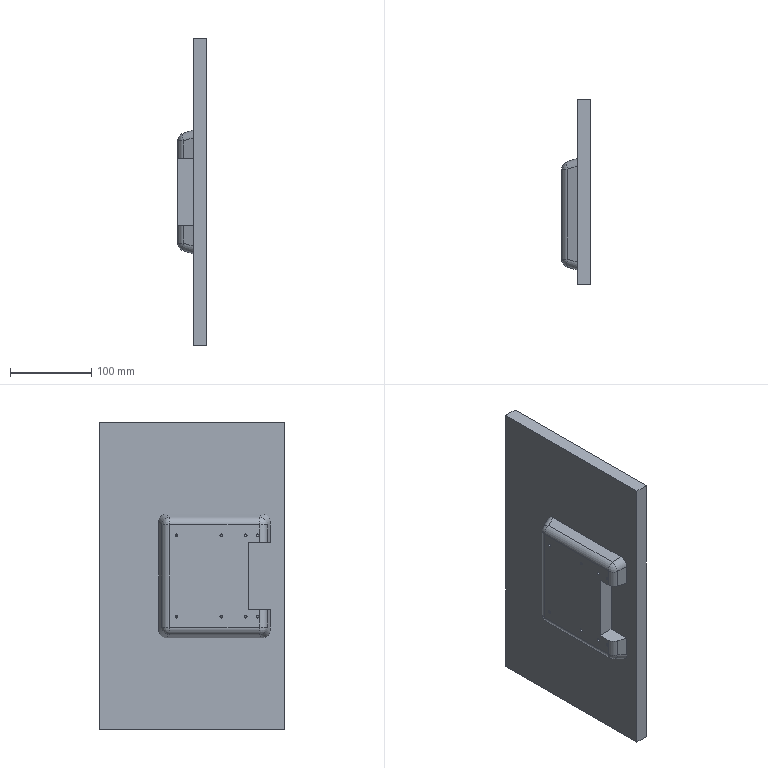Part | NX | 1 solid | 49 faces | box 35 x 228 x 378 mm | volume 1358044 mm3 | plane 20 | cylinder 17 | cone 8 | sphere 4 | commonest cylinder face diameters 20 x9 3.3 x8
STEP:
#1=CARTESIAN_POINT('',(-11.924,-92.355,62.792));
#2=VERTEX_POINT('',#1);
#3=CARTESIAN_POINT('',(-11.924,-92.355,41.5));
#4=VERTEX_POINT('',#3);
#5=CARTESIAN_POINT('',(-11.924,-92.355,-60.628));
#6=DIRECTION('',(0.,0.,1.));
#7=VECTOR('',#6,1000.);
#8=LINE('',#5,#7);
#9=EDGE_CURVE('',#2,#4,#8,.F.);
#10=ORIENTED_EDGE('',*,*,#9,.T.);
#11=CARTESIAN_POINT('',(0.,-96.,41.5));
#12=VERTEX_POINT('',#11);
#13=CARTESIAN_POINT('',(0.,-96.,41.5));
#14=DIRECTION('',(-0.9563,0.2924,0.));
#15=VECTOR('',#14,1000.);
#16=LINE('',#13,#15);
#17=EDGE_CURVE('',#4,#12,#16,.F.);
#18=ORIENTED_EDGE('',*,*,#17,.T.);
#19=CARTESIAN_POINT('',(0.,-96.,66.437));
#20=VERTEX_POINT('',#19);
#21=CARTESIAN_POINT('',(0.,-96.,-76.));
#22=DIRECTION('',(0.,0.,1.));
#23=VECTOR('',#22,1000.);
#24=LINE('',#21,#23);
#25=EDGE_CURVE('',#12,#20,#24,.T.);
#26=ORIENTED_EDGE('',*,*,#25,.T.);
#27=CARTESIAN_POINT('',(-36.689,-84.783,55.22));
#28=DIRECTION('',(-0.9179,0.2806,-0.2806));
#29=VECTOR('',#28,1000.);
#30=LINE('',#27,#29);
#31=EDGE_CURVE('',#20,#2,#30,.T.);
#32=ORIENTED_EDGE('',*,*,#31,.T.);
#33=EDGE_LOOP('',(#10,#18,#26,#32));
#34=FACE_BOUND('',#33,.T.);
#35=CARTESIAN_POINT('',(0.,-96.,-76.));
#36=DIRECTION('',(-0.2924,-0.9563,0.));
#37=DIRECTION('',(0.9563,-0.2924,0.));
#38=AXIS2_PLACEMENT_3D('',#35,#36,#37);
#39=PLANE('',#38);
#40=ADVANCED_FACE('',(#34),#39,.T.);
#41=CARTESIAN_POINT('',(-19.,-82.792,41.5));
#42=VERTEX_POINT('',#41);
#43=CARTESIAN_POINT('',(-9.,-82.792,41.5));
#44=DIRECTION('',(0.,0.,1.));
#45=DIRECTION('',(0.,-1.,0.));
#46=AXIS2_PLACEMENT_3D('',#43,#44,#45);
#47=CIRCLE('',#46,10.);
#48=EDGE_CURVE('',#4,#42,#47,.F.);
#49=ORIENTED_EDGE('',*,*,#48,.F.);
#50=ORIENTED_EDGE('',*,*,#9,.F.);
#51=CARTESIAN_POINT('',(-19.,-82.792,62.792));
#52=VERTEX_POINT('',#51);
#53=CARTESIAN_POINT('',(-9.,-82.792,62.792));
#54=DIRECTION('',(0.,0.,-1.));
#55=DIRECTION('',(0.,1.,0.));
#56=AXIS2_PLACEMENT_3D('',#53,#54,#55);
#57=CIRCLE('',#56,10.);
#58=EDGE_CURVE('',#2,#52,#57,.T.);
#59=ORIENTED_EDGE('',*,*,#58,.T.);
#60=CARTESIAN_POINT('',(-19.,-82.792,60.628));
#61=DIRECTION('',(0.,0.,-1.));
#62=VECTOR('',#61,1000.);
#63=LINE('',#60,#62);
#64=EDGE_CURVE('',#42,#52,#63,.F.);
#65=ORIENTED_EDGE('',*,*,#64,.F.);
#66=EDGE_LOOP('',(#49,#50,#59,#65));
#67=FACE_BOUND('',#66,.T.);
#68=CARTESIAN_POINT('',(-9.,-82.792,0.));
#69=DIRECTION('',(0.,0.,1.));
#70=DIRECTION('',(0.,-1.,0.));
#71=AXIS2_PLACEMENT_3D('',#68,#69,#70);
#72=CYLINDRICAL_SURFACE('',#71,10.);
#73=ADVANCED_FACE('',(#67),#72,.T.);
#74=CARTESIAN_POINT('',(0.,-114.,-189.));
#75=VERTEX_POINT('',#74);
#76=CARTESIAN_POINT('',(0.,114.,-189.));
#77=VERTEX_POINT('',#76);
#78=CARTESIAN_POINT('',(0.,114.,-189.));
#79=DIRECTION('',(0.,1.,0.));
#80=VECTOR('',#79,1000.);
#81=LINE('',#78,#80);
#82=EDGE_CURVE('',#75,#77,#81,.T.);
#83=ORIENTED_EDGE('',*,*,#82,.F.);
#84=CARTESIAN_POINT('',(0.,-114.,189.));
#85=VERTEX_POINT('',#84);
#86=CARTESIAN_POINT('',(0.,-114.,189.));
#87=DIRECTION('',(0.,0.,-1.));
#88=VECTOR('',#87,1000.);
#89=LINE('',#86,#88);
#90=EDGE_CURVE('',#85,#75,#89,.T.);
#91=ORIENTED_EDGE('',*,*,#90,.F.);
#92=CARTESIAN_POINT('',(0.,114.,189.));
#93=VERTEX_POINT('',#92);
#94=CARTESIAN_POINT('',(0.,114.,189.));
#95=DIRECTION('',(0.,-1.,0.));
#96=VECTOR('',#95,1000.);
#97=LINE('',#94,#96);
#98=EDGE_CURVE('',#93,#85,#97,.T.);
#99=ORIENTED_EDGE('',*,*,#98,.F.);
#100=CARTESIAN_POINT('',(0.,114.,189.));
#101=DIRECTION('',(0.,0.,1.));
#102=VECTOR('',#101,1000.);
#103=LINE('',#100,#102);
#104=EDGE_CURVE('',#77,#93,#103,.T.);
#105=ORIENTED_EDGE('',*,*,#104,.F.);
#106=EDGE_LOOP('',(#83,#91,#99,#105));
#107=FACE_BOUND('',#106,.T.);
#108=ORIENTED_EDGE('',*,*,#25,.F.);
#109=CARTESIAN_POINT('',(0.,-69.,41.5));
#110=VERTEX_POINT('',#109);
#111=CARTESIAN_POINT('',(0.,-69.,41.5));
#112=DIRECTION('',(0.,1.,0.));
#113=VECTOR('',#112,1000.);
#114=LINE('',#111,#113);
#115=EDGE_CURVE('',#12,#110,#114,.T.);
#116=ORIENTED_EDGE('',*,*,#115,.T.);
#117=CARTESIAN_POINT('',(0.,-69.,-41.5));
#118=VERTEX_POINT('',#117);
#119=CARTESIAN_POINT('',(0.,-69.,-41.5));
#120=DIRECTION('',(0.,0.,-1.));
#121=VECTOR('',#120,1000.);
#122=LINE('',#119,#121);
#123=EDGE_CURVE('',#110,#118,#122,.T.);
#124=ORIENTED_EDGE('',*,*,#123,.T.);
#125=CARTESIAN_POINT('',(0.,-96.,-41.5));
#126=VERTEX_POINT('',#125);
#127=CARTESIAN_POINT('',(0.,-69.,-41.5));
#128=DIRECTION('',(0.,-1.,0.));
#129=VECTOR('',#128,1000.);
#130=LINE('',#127,#129);
#131=EDGE_CURVE('',#118,#126,#130,.T.);
#132=ORIENTED_EDGE('',*,*,#131,.T.);
#133=CARTESIAN_POINT('',(0.,-96.,-66.437));
#134=VERTEX_POINT('',#133);
#135=CARTESIAN_POINT('',(0.,-96.,-76.));
#136=DIRECTION('',(0.,0.,1.));
#137=VECTOR('',#136,1000.);
#138=LINE('',#135,#137);
#139=EDGE_CURVE('',#134,#126,#138,.T.);
#140=ORIENTED_EDGE('',*,*,#139,.F.);
#141=CARTESIAN_POINT('',(0.,-86.437,-76.));
#142=VERTEX_POINT('',#141);
#143=CARTESIAN_POINT('',(0.,-85.543,-65.543));
#144=DIRECTION('',(1.,0.,0.));
#145=DIRECTION('',(0.,-0.7071,-0.7071));
#146=AXIS2_PLACEMENT_3D('',#143,#144,#145);
#147=ELLIPSE('',#146,10.895,10.);
#148=EDGE_CURVE('',#134,#142,#147,.T.);
#149=ORIENTED_EDGE('',*,*,#148,.T.);
#150=CARTESIAN_POINT('',(0.,31.437,-76.));
#151=VERTEX_POINT('',#150);
#152=CARTESIAN_POINT('',(0.,41.,-76.));
#153=DIRECTION('',(0.,-1.,0.));
#154=VECTOR('',#153,1000.);
#155=LINE('',#152,#154);
#156=EDGE_CURVE('',#151,#142,#155,.T.);
#157=ORIENTED_EDGE('',*,*,#156,.F.);
#158=CARTESIAN_POINT('',(0.,41.,-66.437));
#159=VERTEX_POINT('',#158);
#160=CARTESIAN_POINT('',(0.,30.543,-65.543));
#161=DIRECTION('',(1.,0.,0.));
#162=DIRECTION('',(0.,0.7071,-0.7071));
#163=AXIS2_PLACEMENT_3D('',#160,#161,#162);
#164=ELLIPSE('',#163,10.895,10.);
#165=EDGE_CURVE('',#151,#159,#164,.T.);
#166=ORIENTED_EDGE('',*,*,#165,.T.);
#167=CARTESIAN_POINT('',(0.,41.,66.437));
#168=VERTEX_POINT('',#167);
#169=CARTESIAN_POINT('',(0.,41.,-76.));
#170=DIRECTION('',(0.,0.,-1.));
#171=VECTOR('',#170,1000.);
#172=LINE('',#169,#171);
#173=EDGE_CURVE('',#168,#159,#172,.T.);
#174=ORIENTED_EDGE('',*,*,#173,.F.);
#175=CARTESIAN_POINT('',(0.,31.437,76.));
#176=VERTEX_POINT('',#175);
#177=CARTESIAN_POINT('',(0.,30.543,65.543));
#178=DIRECTION('',(1.,0.,0.));
#179=DIRECTION('',(0.,0.7071,0.7071));
#180=AXIS2_PLACEMENT_3D('',#177,#178,#179);
#181=ELLIPSE('',#180,10.895,10.);
#182=EDGE_CURVE('',#168,#176,#181,.T.);
#183=ORIENTED_EDGE('',*,*,#182,.T.);
#184=CARTESIAN_POINT('',(0.,-86.437,76.));
#185=VERTEX_POINT('',#184);
#186=CARTESIAN_POINT('',(0.,41.,76.));
#187=DIRECTION('',(0.,1.,0.));
#188=VECTOR('',#187,1000.);
#189=LINE('',#186,#188);
#190=EDGE_CURVE('',#185,#176,#189,.T.);
#191=ORIENTED_EDGE('',*,*,#190,.F.);
#192=CARTESIAN_POINT('',(0.,-85.543,65.543));
#193=DIRECTION('',(1.,0.,0.));
#194=DIRECTION('',(0.,-0.7071,0.7071));
#195=AXIS2_PLACEMENT_3D('',#192,#193,#194);
#196=ELLIPSE('',#195,10.895,10.);
#197=EDGE_CURVE('',#185,#20,#196,.T.);
#198=ORIENTED_EDGE('',*,*,#197,.T.);
#199=EDGE_LOOP('',(#108,#116,#124,#132,#140,#149,#157,#166,#174,#183,#191,#198));
#200=FACE_BOUND('',#199,.T.);
#201=CARTESIAN_POINT('',(0.,0.,0.));
#202=DIRECTION('',(1.,0.,0.));
#203=DIRECTION('',(0.,0.,-1.));
#204=AXIS2_PLACEMENT_3D('',#201,#202,#203);
#205=PLANE('',#204);
#206=ADVANCED_FACE('',(#107,#200),#205,.F.);
#207=ORIENTED_EDGE('',*,*,#82,.T.);
#208=CARTESIAN_POINT('',(16.,114.,-189.));
#209=VERTEX_POINT('',#208);
#210=CARTESIAN_POINT('',(16.,114.,-189.));
#211=DIRECTION('',(-1.,0.,0.));
#212=VECTOR('',#211,1000.);
#213=LINE('',#210,#212);
#214=EDGE_CURVE('',#209,#77,#213,.T.);
#215=ORIENTED_EDGE('',*,*,#214,.F.);
#216=CARTESIAN_POINT('',(16.,-114.,-189.));
#217=VERTEX_POINT('',#216);
#218=CARTESIAN_POINT('',(16.,114.,-189.));
#219=DIRECTION('',(0.,1.,0.));
#220=VECTOR('',#219,1000.);
#221=LINE('',#218,#220);
#222=EDGE_CURVE('',#217,#209,#221,.T.);
#223=ORIENTED_EDGE('',*,*,#222,.F.);
#224=CARTESIAN_POINT('',(16.,-114.,-189.));
#225=DIRECTION('',(-1.,0.,0.));
#226=VECTOR('',#225,1000.);
#227=LINE('',#224,#226);
#228=EDGE_CURVE('',#217,#75,#227,.T.);
#229=ORIENTED_EDGE('',*,*,#228,.T.);
#230=EDGE_LOOP('',(#207,#215,#223,#229));
#231=FACE_BOUND('',#230,.T.);
#232=CARTESIAN_POINT('',(16.,114.,-189.));
#233=DIRECTION('',(0.,0.,1.));
#234=DIRECTION('',(0.,-1.,0.));
#235=AXIS2_PLACEMENT_3D('',#232,#233,#234);
#236=PLANE('',#235);
#237=ADVANCED_FACE('',(#231),#236,.F.);
#238=ORIENTED_EDGE('',*,*,#104,.T.);
#239=CARTESIAN_POINT('',(16.,114.,189.));
#240=VERTEX_POINT('',#239);
#241=CARTESIAN_POINT('',(16.,114.,189.));
#242=DIRECTION('',(-1.,0.,0.));
#243=VECTOR('',#242,1000.);
#244=LINE('',#241,#243);
#245=EDGE_CURVE('',#240,#93,#244,.T.);
#246=ORIENTED_EDGE('',*,*,#245,.F.);
#247=CARTESIAN_POINT('',(16.,114.,189.));
#248=DIRECTION('',(0.,0.,1.));
#249=VECTOR('',#248,1000.);
#250=LINE('',#247,#249);
#251=EDGE_CURVE('',#209,#240,#250,.T.);
#252=ORIENTED_EDGE('',*,*,#251,.F.);
#253=ORIENTED_EDGE('',*,*,#214,.T.);
#254=EDGE_LOOP('',(#238,#246,#252,#253));
#255=FACE_BOUND('',#254,.T.);
#256=CARTESIAN_POINT('',(16.,114.,189.));
#257=DIRECTION('',(0.,-1.,0.));
#258=DIRECTION('',(0.,0.,-1.));
#259=AXIS2_PLACEMENT_3D('',#256,#257,#258);
#260=PLANE('',#259);
#261=ADVANCED_FACE('',(#255),#260,.F.);
#262=ORIENTED_EDGE('',*,*,#98,.T.);
#263=CARTESIAN_POINT('',(16.,-114.,189.));
#264=VERTEX_POINT('',#263);
#265=CARTESIAN_POINT('',(16.,-114.,189.));
#266=DIRECTION('',(-1.,0.,0.));
#267=VECTOR('',#266,1000.);
#268=LINE('',#265,#267);
#269=EDGE_CURVE('',#264,#85,#268,.T.);
#270=ORIENTED_EDGE('',*,*,#269,.F.);
#271=CARTESIAN_POINT('',(16.,114.,189.));
#272=DIRECTION('',(0.,-1.,0.));
#273=VECTOR('',#272,1000.);
#274=LINE('',#271,#273);
#275=EDGE_CURVE('',#240,#264,#274,.T.);
#276=ORIENTED_EDGE('',*,*,#275,.F.);
#277=ORIENTED_EDGE('',*,*,#245,.T.);
#278=EDGE_LOOP('',(#262,#270,#276,#277));
#279=FACE_BOUND('',#278,.T.);
#280=CARTESIAN_POINT('',(16.,114.,189.));
#281=DIRECTION('',(0.,0.,-1.));
#282=DIRECTION('',(0.,1.,0.));
#283=AXIS2_PLACEMENT_3D('',#280,#281,#282);
#284=PLANE('',#283);
#285=ADVANCED_FACE('',(#279),#284,.F.);
#286=ORIENTED_EDGE('',*,*,#90,.T.);
#287=ORIENTED_EDGE('',*,*,#228,.F.);
#288=CARTESIAN_POINT('',(16.,-114.,189.));
#289=DIRECTION('',(0.,0.,-1.));
#290=VECTOR('',#289,1000.);
#291=LINE('',#288,#290);
#292=EDGE_CURVE('',#264,#217,#291,.T.);
#293=ORIENTED_EDGE('',*,*,#292,.F.);
#294=ORIENTED_EDGE('',*,*,#269,.T.);
#295=EDGE_LOOP('',(#286,#287,#293,#294));
#296=FACE_BOUND('',#295,.T.);
#297=CARTESIAN_POINT('',(16.,-114.,189.));
#298=DIRECTION('',(0.,1.,0.));
#299=DIRECTION('',(0.,0.,1.));
#300=AXIS2_PLACEMENT_3D('',#297,#298,#299);
#301=PLANE('',#300);
#302=ADVANCED_FACE('',(#296),#301,.F.);
#303=CARTESIAN_POINT('',(16.,-97.,-174.));
#304=VERTEX_POINT('',#303);
#305=CARTESIAN_POINT('',(16.,99.,-174.));
#306=VERTEX_POINT('',#305);
#307=CARTESIAN_POINT('',(16.,99.,-174.));
#308=DIRECTION('',(0.,1.,0.));
#309=VECTOR('',#308,1000.);
#310=LINE('',#307,#309);
#311=EDGE_CURVE('',#304,#306,#310,.T.);
#312=ORIENTED_EDGE('',*,*,#311,.F.);
#313=CARTESIAN_POINT('',(16.,-97.,174.));
#314=VERTEX_POINT('',#313);
#315=CARTESIAN_POINT('',(16.,-97.,174.));
#316=DIRECTION('',(0.,0.,-1.));
#317=VECTOR('',#316,1000.);
#318=LINE('',#315,#317);
#319=EDGE_CURVE('',#314,#304,#318,.T.);
#320=ORIENTED_EDGE('',*,*,#319,.F.);
#321=CARTESIAN_POINT('',(16.,99.,174.));
#322=VERTEX_POINT('',#321);
#323=CARTESIAN_POINT('',(16.,99.,174.));
#324=DIRECTION('',(0.,-1.,0.));
#325=VECTOR('',#324,1000.);
#326=LINE('',#323,#325);
#327=EDGE_CURVE('',#322,#314,#326,.T.);
#328=ORIENTED_EDGE('',*,*,#327,.F.);
#329=CARTESIAN_POINT('',(16.,99.,174.));
#330=DIRECTION('',(0.,0.,1.));
#331=VECTOR('',#330,1000.);
#332=LINE('',#329,#331);
#333=EDGE_CURVE('',#306,#322,#332,.T.);
#334=ORIENTED_EDGE('',*,*,#333,.F.);
#335=EDGE_LOOP('',(#312,#320,#328,#334));
#336=FACE_BOUND('',#335,.T.);
#337=ORIENTED_EDGE('',*,*,#222,.T.);
#338=ORIENTED_EDGE('',*,*,#251,.T.);
#339=ORIENTED_EDGE('',*,*,#275,.T.);
#340=ORIENTED_EDGE('',*,*,#292,.T.);
#341=EDGE_LOOP('',(#337,#338,#339,#340));
#342=FACE_BOUND('',#341,.T.);
#343=CARTESIAN_POINT('',(16.,0.,0.));
#344=DIRECTION('',(1.,0.,0.));
#345=DIRECTION('',(0.,0.,-1.));
#346=AXIS2_PLACEMENT_3D('',#343,#344,#345);
#347=PLANE('',#346);
#348=ADVANCED_FACE('',(#336,#342),#347,.T.);
#349=ORIENTED_EDGE('',*,*,#311,.T.);
#350=CARTESIAN_POINT('',(11.,99.,-174.));
#351=VERTEX_POINT('',#350);
#352=CARTESIAN_POINT('',(11.,99.,-174.));
#353=DIRECTION('',(1.,0.,0.));
#354=VECTOR('',#353,1000.);
#355=LINE('',#352,#354);
#356=EDGE_CURVE('',#351,#306,#355,.T.);
#357=ORIENTED_EDGE('',*,*,#356,.F.);
#358=CARTESIAN_POINT('',(11.,-97.,-174.));
#359=VERTEX_POINT('',#358);
#360=CARTESIAN_POINT('',(11.,99.,-174.));
#361=DIRECTION('',(0.,1.,0.));
#362=VECTOR('',#361,1000.);
#363=LINE('',#360,#362);
#364=EDGE_CURVE('',#359,#351,#363,.T.);
#365=ORIENTED_EDGE('',*,*,#364,.F.);
#366=CARTESIAN_POINT('',(11.,-97.,-174.));
#367=DIRECTION('',(1.,0.,0.));
#368=VECTOR('',#367,1000.);
#369=LINE('',#366,#368);
#370=EDGE_CURVE('',#359,#304,#369,.T.);
#371=ORIENTED_EDGE('',*,*,#370,.T.);
#372=EDGE_LOOP('',(#349,#357,#365,#371));
#373=FACE_BOUND('',#372,.T.);
#374=CARTESIAN_POINT('',(11.,99.,-174.));
#375=DIRECTION('',(0.,0.,-1.));
#376=DIRECTION('',(-1.,0.,0.));
#377=AXIS2_PLACEMENT_3D('',#374,#375,#376);
#378=PLANE('',#377);
#379=ADVANCED_FACE('',(#373),#378,.F.);
#380=ORIENTED_EDGE('',*,*,#319,.T.);
#381=ORIENTED_EDGE('',*,*,#370,.F.);
#382=CARTESIAN_POINT('',(11.,-97.,174.));
#383=VERTEX_POINT('',#382);
#384=CARTESIAN_POINT('',(11.,-97.,174.));
#385=DIRECTION('',(0.,0.,-1.));
#386=VECTOR('',#385,1000.);
#387=LINE('',#384,#386);
#388=EDGE_CURVE('',#383,#359,#387,.T.);
#389=ORIENTED_EDGE('',*,*,#388,.F.);
#390=CARTESIAN_POINT('',(11.,-97.,174.));
#391=DIRECTION('',(1.,0.,0.));
#392=VECTOR('',#391,1000.);
#393=LINE('',#390,#392);
#394=EDGE_CURVE('',#383,#314,#393,.T.);
#395=ORIENTED_EDGE('',*,*,#394,.T.);
#396=EDGE_LOOP('',(#380,#381,#389,#395));
#397=FACE_BOUND('',#396,.T.);
#398=CARTESIAN_POINT('',(11.,-97.,174.));
#399=DIRECTION('',(0.,-1.,0.));
#400=DIRECTION('',(0.,0.,-1.));
#401=AXIS2_PLACEMENT_3D('',#398,#399,#400);
#402=PLANE('',#401);
#403=ADVANCED_FACE('',(#397),#402,.F.);
#404=ORIENTED_EDGE('',*,*,#327,.T.);
#405=ORIENTED_EDGE('',*,*,#394,.F.);
#406=CARTESIAN_POINT('',(11.,99.,174.));
#407=VERTEX_POINT('',#406);
#408=CARTESIAN_POINT('',(11.,99.,174.));
#409=DIRECTION('',(0.,-1.,0.));
#410=VECTOR('',#409,1000.);
#411=LINE('',#408,#410);
#412=EDGE_CURVE('',#407,#383,#411,.T.);
#413=ORIENTED_EDGE('',*,*,#412,.F.);
#414=CARTESIAN_POINT('',(11.,99.,174.));
#415=DIRECTION('',(1.,0.,0.));
#416=VECTOR('',#415,1000.);
#417=LINE('',#414,#416);
#418=EDGE_CURVE('',#407,#322,#417,.T.);
#419=ORIENTED_EDGE('',*,*,#418,.T.);
#420=EDGE_LOOP('',(#404,#405,#413,#419));
#421=FACE_BOUND('',#420,.T.);
#422=CARTESIAN_POINT('',(11.,99.,174.));
#423=DIRECTION('',(0.,0.,1.));
#424=DIRECTION('',(0.,-1.,0.));
#425=AXIS2_PLACEMENT_3D('',#422,#423,#424);
#426=PLANE('',#425);
#427=ADVANCED_FACE('',(#421),#426,.F.);
#428=ORIENTED_EDGE('',*,*,#333,.T.);
#429=ORIENTED_EDGE('',*,*,#418,.F.);
#430=CARTESIAN_POINT('',(11.,99.,174.));
#431=DIRECTION('',(0.,0.,1.));
#432=VECTOR('',#431,1000.);
#433=LINE('',#430,#432);
#434=EDGE_CURVE('',#351,#407,#433,.T.);
#435=ORIENTED_EDGE('',*,*,#434,.F.);
#436=ORIENTED_EDGE('',*,*,#356,.T.);
#437=EDGE_LOOP('',(#428,#429,#435,#436));
#438=FACE_BOUND('',#437,.T.);
#439=CARTESIAN_POINT('',(11.,99.,174.));
#440=DIRECTION('',(0.,1.,0.));
#441=DIRECTION('',(0.,0.,1.));
#442=AXIS2_PLACEMENT_3D('',#439,#440,#441);
#443=PLANE('',#442);
#444=ADVANCED_FACE('',(#438),#443,.F.);
#445=ORIENTED_EDGE('',*,*,#364,.T.);
#446=ORIENTED_EDGE('',*,*,#434,.T.);
#447=ORIENTED_EDGE('',*,*,#412,.T.);
#448=ORIENTED_EDGE('',*,*,#388,.T.);
#449=EDGE_LOOP('',(#445,#446,#447,#448));
#450=FACE_BOUND('',#449,.T.);
#451=CARTESIAN_POINT('',(11.,0.,0.));
#452=DIRECTION('',(1.,0.,0.));
#453=DIRECTION('',(0.,0.,-1.));
#454=AXIS2_PLACEMENT_3D('',#451,#452,#453);
#455=PLANE('',#454);
#456=ADVANCED_FACE('',(#450),#455,.T.);
#457=CARTESIAN_POINT('',(-11.924,27.792,72.355));
#458=VERTEX_POINT('',#457);
#459=CARTESIAN_POINT('',(2.463,32.19,76.753));
#460=DIRECTION('',(-0.9179,-0.2806,-0.2806));
#461=VECTOR('',#460,1000.);
#462=LINE('',#459,#461);
#463=EDGE_CURVE('',#176,#458,#462,.T.);
#464=ORIENTED_EDGE('',*,*,#463,.T.);
#465=CARTESIAN_POINT('',(-11.924,-82.792,72.355));
#466=VERTEX_POINT('',#465);
#467=CARTESIAN_POINT('',(-11.924,-80.628,72.355));
#468=DIRECTION('',(0.,1.,0.));
#469=VECTOR('',#468,1000.);
#470=LINE('',#467,#469);
#471=EDGE_CURVE('',#458,#466,#470,.F.);
#472=ORIENTED_EDGE('',*,*,#471,.T.);
#473=CARTESIAN_POINT('',(-32.825,-76.401,65.964));
#474=DIRECTION('',(-0.9179,0.2806,-0.2806));
#475=VECTOR('',#474,1000.);
#476=LINE('',#473,#475);
#477=EDGE_CURVE('',#466,#185,#476,.F.);
#478=ORIENTED_EDGE('',*,*,#477,.T.);
#479=ORIENTED_EDGE('',*,*,#190,.T.);
#480=EDGE_LOOP('',(#464,#472,#478,#479));
#481=FACE_BOUND('',#480,.T.);
#482=CARTESIAN_POINT('',(0.,41.,76.));
#483=DIRECTION('',(-0.2924,0.,0.9563));
#484=DIRECTION('',(0.9563,0.,0.2924));
#485=AXIS2_PLACEMENT_3D('',#482,#483,#484);
#486=PLANE('',#485);
#487=ADVANCED_FACE('',(#481),#486,.T.);
#488=CARTESIAN_POINT('',(-11.924,37.355,-62.792));
#489=VERTEX_POINT('',#488);
#490=CARTESIAN_POINT('',(2.463,41.753,-67.19));
#491=DIRECTION('',(-0.9179,-0.2806,0.2806));
#492=VECTOR('',#491,1000.);
#493=LINE('',#490,#492);
#494=EDGE_CURVE('',#159,#489,#493,.T.);
#495=ORIENTED_EDGE('',*,*,#494,.T.);
#496=CARTESIAN_POINT('',(-11.924,37.355,62.792));
#497=VERTEX_POINT('',#496);
#498=CARTESIAN_POINT('',(-11.924,37.355,60.628));
#499=DIRECTION('',(0.,0.,-1.));
#500=VECTOR('',#499,1000.);
#501=LINE('',#498,#500);
#502=EDGE_CURVE('',#489,#497,#501,.F.);
#503=ORIENTED_EDGE('',*,*,#502,.T.);
#504=CARTESIAN_POINT('',(-36.689,29.783,55.22));
#505=DIRECTION('',(-0.9179,-0.2806,-0.2806));
#506=VECTOR('',#505,1000.);
#507=LINE('',#504,#506);
#508=EDGE_CURVE('',#497,#168,#507,.F.);
#509=ORIENTED_EDGE('',*,*,#508,.T.);
#510=ORIENTED_EDGE('',*,*,#173,.T.);
#511=EDGE_LOOP('',(#495,#503,#509,#510));
#512=FACE_BOUND('',#511,.T.);
#513=CARTESIAN_POINT('',(0.,41.,-76.));
#514=DIRECTION('',(-0.2924,0.9563,0.));
#515=DIRECTION('',(-0.9563,-0.2924,0.));
#516=AXIS2_PLACEMENT_3D('',#513,#514,#515);
#517=PLANE('',#516);
#518=ADVANCED_FACE('',(#512),#517,.T.);
#519=CARTESIAN_POINT('',(-11.924,-82.792,-72.355));
#520=VERTEX_POINT('',#519);
#521=CARTESIAN_POINT('',(-32.825,-76.401,-65.964));
#522=DIRECTION('',(-0.9179,0.2806,0.2806));
#523=VECTOR('',#522,1000.);
#524=LINE('',#521,#523);
#525=EDGE_CURVE('',#142,#520,#524,.T.);
#526=ORIENTED_EDGE('',*,*,#525,.T.);
#527=CARTESIAN_POINT('',(-11.924,27.792,-72.355));
#528=VERTEX_POINT('',#527);
#529=CARTESIAN_POINT('',(-11.924,25.628,-72.355));
#530=DIRECTION('',(0.,-1.,0.));
#531=VECTOR('',#530,1000.);
#532=LINE('',#529,#531);
#533=EDGE_CURVE('',#520,#528,#532,.F.);
#534=ORIENTED_EDGE('',*,*,#533,.T.);
#535=CARTESIAN_POINT('',(2.463,32.19,-76.753));
#536=DIRECTION('',(-0.9179,-0.2806,0.2806));
#537=VECTOR('',#536,1000.);
#538=LINE('',#535,#537);
#539=EDGE_CURVE('',#528,#151,#538,.F.);
#540=ORIENTED_EDGE('',*,*,#539,.T.);
#541=ORIENTED_EDGE('',*,*,#156,.T.);
#542=EDGE_LOOP('',(#526,#534,#540,#541));
#543=FACE_BOUND('',#542,.T.);
#544=CARTESIAN_POINT('',(0.,41.,-76.));
#545=DIRECTION('',(-0.2924,0.,-0.9563));
#546=DIRECTION('',(-0.9563,0.,0.2924));
#547=AXIS2_PLACEMENT_3D('',#544,#545,#546);
#548=PLANE('',#547);
#549=ADVANCED_FACE('',(#543),#548,.T.);
#550=ORIENTED_EDGE('',*,*,#139,.T.);
#551=CARTESIAN_POINT('',(-11.924,-92.355,-41.5));
#552=VERTEX_POINT('',#551);
#553=CARTESIAN_POINT('',(0.,-96.,-41.5));
#554=DIRECTION('',(0.9563,-0.2924,0.));
#555=VECTOR('',#554,1000.);
#556=LINE('',#553,#555);
#557=EDGE_CURVE('',#126,#552,#556,.F.);
#558=ORIENTED_EDGE('',*,*,#557,.T.);
#559=CARTESIAN_POINT('',(-11.924,-92.355,-62.792));
#560=VERTEX_POINT('',#559);
#561=CARTESIAN_POINT('',(-11.924,-92.355,-60.628));
#562=DIRECTION('',(0.,0.,1.));
#563=VECTOR('',#562,1000.);
#564=LINE('',#561,#563);
#565=EDGE_CURVE('',#552,#560,#564,.F.);
#566=ORIENTED_EDGE('',*,*,#565,.T.);
#567=CARTESIAN_POINT('',(2.463,-96.753,-67.19));
#568=DIRECTION('',(-0.9179,0.2806,0.2806));
#569=VECTOR('',#568,1000.);
#570=LINE('',#567,#569);
#571=EDGE_CURVE('',#560,#134,#570,.F.);
#572=ORIENTED_EDGE('',*,*,#571,.T.);
#573=EDGE_LOOP('',(#550,#558,#566,#572));
#574=FACE_BOUND('',#573,.T.);
#575=CARTESIAN_POINT('',(0.,-96.,-76.));
#576=DIRECTION('',(-0.2924,-0.9563,0.));
#577=DIRECTION('',(0.9563,-0.2924,0.));
#578=AXIS2_PLACEMENT_3D('',#575,#576,#577);
#579=PLANE('',#578);
#580=ADVANCED_FACE('',(#574),#579,.T.);
#581=CARTESIAN_POINT('',(-19.,-81.,51.65));
#582=VERTEX_POINT('',#581);
#583=CARTESIAN_POINT('',(-19.,-81.,50.));
#584=DIRECTION('',(-1.,0.,0.));
#585=DIRECTION('',(0.,0.,1.));
#586=AXIS2_PLACEMENT_3D('',#583,#584,#585);
#587=CIRCLE('',#586,1.65);
#588=EDGE_CURVE('',#582,#582,#587,.T.);
#589=ORIENTED_EDGE('',*,*,#588,.F.);
#590=EDGE_LOOP('',(#589));
#591=FACE_BOUND('',#590,.T.);
#592=CARTESIAN_POINT('',(-19.,-81.,-48.35));
#593=VERTEX_POINT('',#592);
#594=CARTESIAN_POINT('',(-19.,-81.,-50.));
#595=DIRECTION('',(-1.,0.,0.));
#596=DIRECTION('',(0.,0.,1.));
#597=AXIS2_PLACEMENT_3D('',#594,#595,#596);
#598=CIRCLE('',#597,1.65);
#599=EDGE_CURVE('',#593,#593,#598,.T.);
#600=ORIENTED_EDGE('',*,*,#599,.F.);
#601=EDGE_LOOP('',(#600));
#602=FACE_BOUND('',#601,.T.);
#603=CARTESIAN_POINT('',(-19.,-66.,-48.35));
#604=VERTEX_POINT('',#603);
#605=CARTESIAN_POINT('',(-19.,-66.,-50.));
#606=DIRECTION('',(-1.,0.,0.));
#607=DIRECTION('',(0.,0.,1.));
#608=AXIS2_PLACEMENT_3D('',#605,#606,#607);
#609=CIRCLE('',#608,1.65);
#610=EDGE_CURVE('',#604,#604,#609,.T.);
#611=ORIENTED_EDGE('',*,*,#610,.F.);
#612=EDGE_LOOP('',(#611));
#613=FACE_BOUND('',#612,.T.);
#614=CARTESIAN_POINT('',(-19.,-66.,51.65));
#615=VERTEX_POINT('',#614);
#616=CARTESIAN_POINT('',(-19.,-66.,50.));
#617=DIRECTION('',(-1.,0.,0.));
#618=DIRECTION('',(0.,0.,1.));
#619=AXIS2_PLACEMENT_3D('',#616,#617,#618);
#620=CIRCLE('',#619,1.65);
#621=EDGE_CURVE('',#615,#615,#620,.T.);
#622=ORIENTED_EDGE('',*,*,#621,.F.);
#623=EDGE_LOOP('',(#622));
#624=FACE_BOUND('',#623,.T.);
#625=CARTESIAN_POINT('',(-19.,-36.,-48.35));
#626=VERTEX_POINT('',#625);
#627=CARTESIAN_POINT('',(-19.,-36.,-50.));
#628=DIRECTION('',(-1.,0.,0.));
#629=DIRECTION('',(0.,0.,1.));
#630=AXIS2_PLACEMENT_3D('',#627,#628,#629);
#631=CIRCLE('',#630,1.65);
#632=EDGE_CURVE('',#626,#626,#631,.T.);
#633=ORIENTED_EDGE('',*,*,#632,.F.);
#634=EDGE_LOOP('',(#633));
#635=FACE_BOUND('',#634,.T.);
#636=CARTESIAN_POINT('',(-19.,-36.,51.65));
#637=VERTEX_POINT('',#636);
#638=CARTESIAN_POINT('',(-19.,-36.,50.));
#639=DIRECTION('',(-1.,0.,0.));
#640=DIRECTION('',(0.,0.,1.));
#641=AXIS2_PLACEMENT_3D('',#638,#639,#640);
#642=CIRCLE('',#641,1.65);
#643=EDGE_CURVE('',#637,#637,#642,.T.);
#644=ORIENTED_EDGE('',*,*,#643,.F.);
#645=EDGE_LOOP('',(#644));
#646=FACE_BOUND('',#645,.T.);
#647=CARTESIAN_POINT('',(-19.,19.,-48.35));
#648=VERTEX_POINT('',#647);
#649=CARTESIAN_POINT('',(-19.,19.,-50.));
#650=DIRECTION('',(-1.,0.,0.));
#651=DIRECTION('',(0.,0.,1.));
#652=AXIS2_PLACEMENT_3D('',#649,#650,#651);
#653=CIRCLE('',#652,1.65);
#654=EDGE_CURVE('',#648,#648,#653,.T.);
#655=ORIENTED_EDGE('',*,*,#654,.F.);
#656=EDGE_LOOP('',(#655));
#657=FACE_BOUND('',#656,.T.);
#658=CARTESIAN_POINT('',(-19.,19.,51.65));
#659=VERTEX_POINT('',#658);
#660=CARTESIAN_POINT('',(-19.,19.,50.));
#661=DIRECTION('',(-1.,0.,0.));
#662=DIRECTION('',(0.,0.,1.));
#663=AXIS2_PLACEMENT_3D('',#660,#661,#662);
#664=CIRCLE('',#663,1.65);
#665=EDGE_CURVE('',#659,#659,#664,.T.);
#666=ORIENTED_EDGE('',*,*,#665,.F.);
#667=EDGE_LOOP('',(#666));
#668=FACE_BOUND('',#667,.T.);
#669=CARTESIAN_POINT('',(-19.,-69.,41.5));
#670=VERTEX_POINT('',#669);
#671=CARTESIAN_POINT('',(-19.,-69.,41.5));
#672=DIRECTION('',(0.,1.,0.));
#673=VECTOR('',#672,1000.);
#674=LINE('',#671,#673);
#675=EDGE_CURVE('',#42,#670,#674,.T.);
#676=ORIENTED_EDGE('',*,*,#675,.F.);
#677=ORIENTED_EDGE('',*,*,#64,.T.);
#678=CARTESIAN_POINT('',(-19.,27.792,62.792));
#679=VERTEX_POINT('',#678);
#680=CARTESIAN_POINT('',(-19.,25.628,62.792));
#681=DIRECTION('',(0.,-1.,0.));
#682=VECTOR('',#681,1000.);
#683=LINE('',#680,#682);
#684=EDGE_CURVE('',#52,#679,#683,.F.);
#685=ORIENTED_EDGE('',*,*,#684,.T.);
#686=CARTESIAN_POINT('',(-19.,27.792,-62.792));
#687=VERTEX_POINT('',#686);
#688=CARTESIAN_POINT('',(-19.,27.792,-60.628));
#689=DIRECTION('',(0.,0.,1.));
#690=VECTOR('',#689,1000.);
#691=LINE('',#688,#690);
#692=EDGE_CURVE('',#679,#687,#691,.F.);
#693=ORIENTED_EDGE('',*,*,#692,.T.);
#694=CARTESIAN_POINT('',(-19.,-82.792,-62.792));
#695=VERTEX_POINT('',#694);
#696=CARTESIAN_POINT('',(-19.,-80.628,-62.792));
#697=DIRECTION('',(0.,1.,0.));
#698=VECTOR('',#697,1000.);
#699=LINE('',#696,#698);
#700=EDGE_CURVE('',#687,#695,#699,.F.);
#701=ORIENTED_EDGE('',*,*,#700,.T.);
#702=CARTESIAN_POINT('',(-19.,-82.792,-41.5));
#703=VERTEX_POINT('',#702);
#704=CARTESIAN_POINT('',(-19.,-82.792,60.628));
#705=DIRECTION('',(0.,0.,-1.));
#706=VECTOR('',#705,1000.);
#707=LINE('',#704,#706);
#708=EDGE_CURVE('',#695,#703,#707,.F.);
#709=ORIENTED_EDGE('',*,*,#708,.T.);
#710=CARTESIAN_POINT('',(-19.,-69.,-41.5));
#711=VERTEX_POINT('',#710);
#712=CARTESIAN_POINT('',(-19.,-69.,-41.5));
#713=DIRECTION('',(0.,-1.,0.));
#714=VECTOR('',#713,1000.);
#715=LINE('',#712,#714);
#716=EDGE_CURVE('',#711,#703,#715,.T.);
#717=ORIENTED_EDGE('',*,*,#716,.F.);
#718=CARTESIAN_POINT('',(-19.,-69.,-41.5));
#719=DIRECTION('',(0.,0.,-1.));
#720=VECTOR('',#719,1000.);
#721=LINE('',#718,#720);
#722=EDGE_CURVE('',#670,#711,#721,.T.);
#723=ORIENTED_EDGE('',*,*,#722,.F.);
#724=EDGE_LOOP('',(#676,#677,#685,#693,#701,#709,#717,#723));
#725=FACE_BOUND('',#724,.T.);
#726=CARTESIAN_POINT('',(-19.,0.,0.));
#727=DIRECTION('',(-1.,0.,0.));
#728=DIRECTION('',(0.,0.,1.));
#729=AXIS2_PLACEMENT_3D('',#726,#727,#728);
#730=PLANE('',#729);
#731=ADVANCED_FACE('',(#591,#602,#613,#624,#635,#646,#657,#668,#725),#730,.T.);
#732=ORIENTED_EDGE('',*,*,#539,.F.);
#733=CARTESIAN_POINT('',(-9.,27.792,-62.792));
#734=DIRECTION('',(0.9179,0.2806,-0.2806));
#735=DIRECTION('',(-0.2924,0.,-0.9563));
#736=AXIS2_PLACEMENT_3D('',#733,#734,#735);
#737=CIRCLE('',#736,10.);
#738=EDGE_CURVE('',#528,#489,#737,.T.);
#739=ORIENTED_EDGE('',*,*,#738,.T.);
#740=ORIENTED_EDGE('',*,*,#494,.F.);
#741=ORIENTED_EDGE('',*,*,#165,.F.);
#742=EDGE_LOOP('',(#732,#739,#740,#741));
#743=FACE_BOUND('',#742,.T.);
#744=CARTESIAN_POINT('',(5.387,32.19,-67.19));
#745=DIRECTION('',(0.9179,0.2806,-0.2806));
#746=DIRECTION('',(-0.2924,0.,-0.9563));
#747=AXIS2_PLACEMENT_3D('',#744,#745,#746);
#748=CYLINDRICAL_SURFACE('',#747,10.);
#749=ADVANCED_FACE('',(#743),#748,.T.);
#750=ORIENTED_EDGE('',*,*,#508,.F.);
#751=CARTESIAN_POINT('',(-9.,27.792,62.792));
#752=DIRECTION('',(0.9179,0.2806,0.2806));
#753=DIRECTION('',(-0.2924,0.9563,0.));
#754=AXIS2_PLACEMENT_3D('',#751,#752,#753);
#755=CIRCLE('',#754,10.);
#756=EDGE_CURVE('',#497,#458,#755,.T.);
#757=ORIENTED_EDGE('',*,*,#756,.T.);
#758=ORIENTED_EDGE('',*,*,#463,.F.);
#759=ORIENTED_EDGE('',*,*,#182,.F.);
#760=EDGE_LOOP('',(#750,#757,#758,#759));
#761=FACE_BOUND('',#760,.T.);
#762=CARTESIAN_POINT('',(-33.765,20.22,55.22));
#763=DIRECTION('',(0.9179,0.2806,0.2806));
#764=DIRECTION('',(-0.2924,0.9563,0.));
#765=AXIS2_PLACEMENT_3D('',#762,#763,#764);
#766=CYLINDRICAL_SURFACE('',#765,10.);
#767=ADVANCED_FACE('',(#761),#766,.T.);
#768=ORIENTED_EDGE('',*,*,#477,.F.);
#769=CARTESIAN_POINT('',(-9.,-82.792,62.792));
#770=DIRECTION('',(0.9179,-0.2806,0.2806));
#771=DIRECTION('',(0.2924,0.,-0.9563));
#772=AXIS2_PLACEMENT_3D('',#769,#770,#771);
#773=CIRCLE('',#772,10.);
#774=EDGE_CURVE('',#466,#2,#773,.T.);
#775=ORIENTED_EDGE('',*,*,#774,.T.);
#776=ORIENTED_EDGE('',*,*,#31,.F.);
#777=ORIENTED_EDGE('',*,*,#197,.F.);
#778=EDGE_LOOP('',(#768,#775,#776,#777));
#779=FACE_BOUND('',#778,.T.);
#780=CARTESIAN_POINT('',(-29.901,-76.401,56.401));
#781=DIRECTION('',(0.9179,-0.2806,0.2806));
#782=DIRECTION('',(0.2924,0.,-0.9563));
#783=AXIS2_PLACEMENT_3D('',#780,#781,#782);
#784=CYLINDRICAL_SURFACE('',#783,10.);
#785=ADVANCED_FACE('',(#779),#784,.T.);
#786=ORIENTED_EDGE('',*,*,#571,.F.);
#787=CARTESIAN_POINT('',(-9.,-82.792,-62.792));
#788=DIRECTION('',(0.9179,-0.2806,-0.2806));
#789=DIRECTION('',(0.2924,0.9563,0.));
#790=AXIS2_PLACEMENT_3D('',#787,#788,#789);
#791=CIRCLE('',#790,10.);
#792=EDGE_CURVE('',#560,#520,#791,.T.);
#793=ORIENTED_EDGE('',*,*,#792,.T.);
#794=ORIENTED_EDGE('',*,*,#525,.F.);
#795=ORIENTED_EDGE('',*,*,#148,.F.);
#796=EDGE_LOOP('',(#786,#793,#794,#795));
#797=FACE_BOUND('',#796,.T.);
#798=CARTESIAN_POINT('',(5.387,-87.19,-67.19));
#799=DIRECTION('',(0.9179,-0.2806,-0.2806));
#800=DIRECTION('',(0.2924,0.9563,0.));
#801=AXIS2_PLACEMENT_3D('',#798,#799,#800);
#802=CYLINDRICAL_SURFACE('',#801,10.);
#803=ADVANCED_FACE('',(#797),#802,.T.);
#804=CARTESIAN_POINT('',(-9.,-82.792,62.792));
#805=DIRECTION('',(0.,-1.,0.));
#806=DIRECTION('',(0.,0.,-1.));
#807=AXIS2_PLACEMENT_3D('',#804,#805,#806);
#808=CIRCLE('',#807,10.);
#809=EDGE_CURVE('',#466,#52,#808,.T.);
#810=ORIENTED_EDGE('',*,*,#809,.F.);
#811=ORIENTED_EDGE('',*,*,#471,.F.);
#812=CARTESIAN_POINT('',(-9.,27.792,62.792));
#813=DIRECTION('',(0.,1.,0.));
#814=DIRECTION('',(0.,0.,1.));
#815=AXIS2_PLACEMENT_3D('',#812,#813,#814);
#816=CIRCLE('',#815,10.);
#817=EDGE_CURVE('',#679,#458,#816,.T.);
#818=ORIENTED_EDGE('',*,*,#817,.F.);
#819=ORIENTED_EDGE('',*,*,#684,.F.);
#820=EDGE_LOOP('',(#810,#811,#818,#819));
#821=FACE_BOUND('',#820,.T.);
#822=CARTESIAN_POINT('',(-9.,0.,62.792));
#823=DIRECTION('',(0.,1.,0.));
#824=DIRECTION('',(0.,0.,1.));
#825=AXIS2_PLACEMENT_3D('',#822,#823,#824);
#826=CYLINDRICAL_SURFACE('',#825,10.);
#827=ADVANCED_FACE('',(#821),#826,.T.);
#828=ORIENTED_EDGE('',*,*,#817,.T.);
#829=ORIENTED_EDGE('',*,*,#756,.F.);
#830=CARTESIAN_POINT('',(-9.,27.792,62.792));
#831=DIRECTION('',(0.,0.,-1.));
#832=DIRECTION('',(0.,1.,0.));
#833=AXIS2_PLACEMENT_3D('',#830,#831,#832);
#834=CIRCLE('',#833,10.);
#835=EDGE_CURVE('',#679,#497,#834,.T.);
#836=ORIENTED_EDGE('',*,*,#835,.F.);
#837=EDGE_LOOP('',(#828,#829,#836));
#838=FACE_BOUND('',#837,.T.);
#839=CARTESIAN_POINT('',(-9.,27.792,62.792));
#840=DIRECTION('',(0.,0.,1.));
#841=DIRECTION('',(1.,0.,0.));
#842=AXIS2_PLACEMENT_3D('',#839,#840,#841);
#843=SPHERICAL_SURFACE('',#842,10.);
#844=ADVANCED_FACE('',(#838),#843,.T.);
#845=ORIENTED_EDGE('',*,*,#774,.F.);
#846=ORIENTED_EDGE('',*,*,#809,.T.);
#847=ORIENTED_EDGE('',*,*,#58,.F.);
#848=EDGE_LOOP('',(#845,#846,#847));
#849=FACE_BOUND('',#848,.T.);
#850=CARTESIAN_POINT('',(-9.,-82.792,62.792));
#851=DIRECTION('',(0.,0.,1.));
#852=DIRECTION('',(1.,0.,0.));
#853=AXIS2_PLACEMENT_3D('',#850,#851,#852);
#854=SPHERICAL_SURFACE('',#853,10.);
#855=ADVANCED_FACE('',(#849),#854,.T.);
#856=ORIENTED_EDGE('',*,*,#835,.T.);
#857=ORIENTED_EDGE('',*,*,#502,.F.);
#858=CARTESIAN_POINT('',(-9.,27.792,-62.792));
#859=DIRECTION('',(0.,0.,-1.));
#860=DIRECTION('',(-1.,0.,0.));
#861=AXIS2_PLACEMENT_3D('',#858,#859,#860);
#862=CIRCLE('',#861,10.);
#863=EDGE_CURVE('',#687,#489,#862,.T.);
#864=ORIENTED_EDGE('',*,*,#863,.F.);
#865=ORIENTED_EDGE('',*,*,#692,.F.);
#866=EDGE_LOOP('',(#856,#857,#864,#865));
#867=FACE_BOUND('',#866,.T.);
#868=CARTESIAN_POINT('',(-9.,27.792,0.));
#869=DIRECTION('',(0.,0.,-1.));
#870=DIRECTION('',(-1.,0.,0.));
#871=AXIS2_PLACEMENT_3D('',#868,#869,#870);
#872=CYLINDRICAL_SURFACE('',#871,10.);
#873=ADVANCED_FACE('',(#867),#872,.T.);
#874=CARTESIAN_POINT('',(-9.,-82.792,-41.5));
#875=DIRECTION('',(0.,0.,-1.));
#876=DIRECTION('',(0.,1.,0.));
#877=AXIS2_PLACEMENT_3D('',#874,#875,#876);
#878=CIRCLE('',#877,10.);
#879=EDGE_CURVE('',#703,#552,#878,.F.);
#880=ORIENTED_EDGE('',*,*,#879,.F.);
#881=ORIENTED_EDGE('',*,*,#708,.F.);
#882=CARTESIAN_POINT('',(-9.,-82.792,-62.792));
#883=DIRECTION('',(0.,0.,-1.));
#884=DIRECTION('',(-1.,0.,0.));
#885=AXIS2_PLACEMENT_3D('',#882,#883,#884);
#886=CIRCLE('',#885,10.);
#887=EDGE_CURVE('',#560,#695,#886,.T.);
#888=ORIENTED_EDGE('',*,*,#887,.F.);
#889=ORIENTED_EDGE('',*,*,#565,.F.);
#890=EDGE_LOOP('',(#880,#881,#888,#889));
#891=FACE_BOUND('',#890,.T.);
#892=CARTESIAN_POINT('',(-9.,-82.792,0.));
#893=DIRECTION('',(0.,0.,1.));
#894=DIRECTION('',(0.,-1.,0.));
#895=AXIS2_PLACEMENT_3D('',#892,#893,#894);
#896=CYLINDRICAL_SURFACE('',#895,10.);
#897=ADVANCED_FACE('',(#891),#896,.T.);
#898=ORIENTED_EDGE('',*,*,#863,.T.);
#899=ORIENTED_EDGE('',*,*,#738,.F.);
#900=CARTESIAN_POINT('',(-9.,27.792,-62.792));
#901=DIRECTION('',(0.,-1.,0.));
#902=DIRECTION('',(0.,0.,-1.));
#903=AXIS2_PLACEMENT_3D('',#900,#901,#902);
#904=CIRCLE('',#903,10.);
#905=EDGE_CURVE('',#687,#528,#904,.T.);
#906=ORIENTED_EDGE('',*,*,#905,.F.);
#907=EDGE_LOOP('',(#898,#899,#906));
#908=FACE_BOUND('',#907,.T.);
#909=CARTESIAN_POINT('',(-9.,27.792,-62.792));
#910=DIRECTION('',(0.,0.,1.));
#911=DIRECTION('',(1.,0.,0.));
#912=AXIS2_PLACEMENT_3D('',#909,#910,#911);
#913=SPHERICAL_SURFACE('',#912,10.);
#914=ADVANCED_FACE('',(#908),#913,.T.);
#915=ORIENTED_EDGE('',*,*,#792,.F.);
#916=ORIENTED_EDGE('',*,*,#887,.T.);
#917=CARTESIAN_POINT('',(-9.,-82.792,-62.792));
#918=DIRECTION('',(0.,1.,0.));
#919=DIRECTION('',(0.,0.,1.));
#920=AXIS2_PLACEMENT_3D('',#917,#918,#919);
#921=CIRCLE('',#920,10.);
#922=EDGE_CURVE('',#520,#695,#921,.T.);
#923=ORIENTED_EDGE('',*,*,#922,.F.);
#924=EDGE_LOOP('',(#915,#916,#923));
#925=FACE_BOUND('',#924,.T.);
#926=CARTESIAN_POINT('',(-9.,-82.792,-62.792));
#927=DIRECTION('',(0.,0.,1.));
#928=DIRECTION('',(1.,0.,0.));
#929=AXIS2_PLACEMENT_3D('',#926,#927,#928);
#930=SPHERICAL_SURFACE('',#929,10.);
#931=ADVANCED_FACE('',(#925),#930,.T.);
#932=ORIENTED_EDGE('',*,*,#905,.T.);
#933=ORIENTED_EDGE('',*,*,#533,.F.);
#934=ORIENTED_EDGE('',*,*,#922,.T.);
#935=ORIENTED_EDGE('',*,*,#700,.F.);
#936=EDGE_LOOP('',(#932,#933,#934,#935));
#937=FACE_BOUND('',#936,.T.);
#938=CARTESIAN_POINT('',(-9.,0.,-62.792));
#939=DIRECTION('',(0.,-1.,0.));
#940=DIRECTION('',(0.,0.,-1.));
#941=AXIS2_PLACEMENT_3D('',#938,#939,#940);
#942=CYLINDRICAL_SURFACE('',#941,10.);
#943=ADVANCED_FACE('',(#937),#942,.T.);
#944=ORIENTED_EDGE('',*,*,#48,.T.);
#945=ORIENTED_EDGE('',*,*,#675,.T.);
#946=CARTESIAN_POINT('',(0.,-69.,41.5));
#947=DIRECTION('',(-1.,0.,0.));
#948=VECTOR('',#947,1000.);
#949=LINE('',#946,#948);
#950=EDGE_CURVE('',#110,#670,#949,.T.);
#951=ORIENTED_EDGE('',*,*,#950,.F.);
#952=ORIENTED_EDGE('',*,*,#115,.F.);
#953=ORIENTED_EDGE('',*,*,#17,.F.);
#954=EDGE_LOOP('',(#944,#945,#951,#952,#953));
#955=FACE_BOUND('',#954,.T.);
#956=CARTESIAN_POINT('',(0.,-69.,41.5));
#957=DIRECTION('',(0.,0.,1.));
#958=DIRECTION('',(0.,-1.,0.));
#959=AXIS2_PLACEMENT_3D('',#956,#957,#958);
#960=PLANE('',#959);
#961=ADVANCED_FACE('',(#955),#960,.F.);
#962=ORIENTED_EDGE('',*,*,#131,.F.);
#963=CARTESIAN_POINT('',(0.,-69.,-41.5));
#964=DIRECTION('',(-1.,0.,0.));
#965=VECTOR('',#964,1000.);
#966=LINE('',#963,#965);
#967=EDGE_CURVE('',#118,#711,#966,.T.);
#968=ORIENTED_EDGE('',*,*,#967,.T.);
#969=ORIENTED_EDGE('',*,*,#716,.T.);
#970=ORIENTED_EDGE('',*,*,#879,.T.);
#971=ORIENTED_EDGE('',*,*,#557,.F.);
#972=EDGE_LOOP('',(#962,#968,#969,#970,#971));
#973=FACE_BOUND('',#972,.T.);
#974=CARTESIAN_POINT('',(0.,-69.,-41.5));
#975=DIRECTION('',(0.,0.,-1.));
#976=DIRECTION('',(0.,1.,0.));
#977=AXIS2_PLACEMENT_3D('',#974,#975,#976);
#978=PLANE('',#977);
#979=ADVANCED_FACE('',(#973),#978,.F.);
#980=ORIENTED_EDGE('',*,*,#722,.T.);
#981=ORIENTED_EDGE('',*,*,#967,.F.);
#982=ORIENTED_EDGE('',*,*,#123,.F.);
#983=ORIENTED_EDGE('',*,*,#950,.T.);
#984=EDGE_LOOP('',(#980,#981,#982,#983));
#985=FACE_BOUND('',#984,.T.);
#986=CARTESIAN_POINT('',(0.,-69.,-41.5));
#987=DIRECTION('',(0.,1.,0.));
#988=DIRECTION('',(0.,0.,1.));
#989=AXIS2_PLACEMENT_3D('',#986,#987,#988);
#990=PLANE('',#989);
#991=ADVANCED_FACE('',(#985),#990,.F.);
#992=CARTESIAN_POINT('',(-7.909,19.,50.));
#993=VERTEX_POINT('',#992);
#994=VERTEX_LOOP('',#993);
#995=FACE_BOUND('',#994,.T.);
#996=CARTESIAN_POINT('',(-8.9,19.,51.65));
#997=VERTEX_POINT('',#996);
#998=CARTESIAN_POINT('',(-8.9,19.,50.));
#999=DIRECTION('',(-1.,0.,0.));
#1000=DIRECTION('',(0.,0.,1.));
#1001=AXIS2_PLACEMENT_3D('',#998,#999,#1000);
#1002=CIRCLE('',#1001,1.65);
#1003=EDGE_CURVE('',#997,#997,#1002,.T.);
#1004=ORIENTED_EDGE('',*,*,#1003,.T.);
#1005=EDGE_LOOP('',(#1004));
#1006=FACE_BOUND('',#1005,.T.);
#1007=CARTESIAN_POINT('',(-8.9,19.,50.));
#1008=DIRECTION('',(-1.,0.,0.));
#1009=DIRECTION('',(0.,0.,1.));
#1010=AXIS2_PLACEMENT_3D('',#1007,#1008,#1009);
#1011=CONICAL_SURFACE('',#1010,1.65,1.03);
#1012=ADVANCED_FACE('',(#995,#1006),#1011,.F.);
#1013=ORIENTED_EDGE('',*,*,#1003,.F.);
#1014=EDGE_LOOP('',(#1013));
#1015=FACE_BOUND('',#1014,.T.);
#1016=ORIENTED_EDGE('',*,*,#665,.T.);
#1017=EDGE_LOOP('',(#1016));
#1018=FACE_BOUND('',#1017,.T.);
#1019=CARTESIAN_POINT('',(-19.,19.,50.));
#1020=DIRECTION('',(-1.,0.,0.));
#1021=DIRECTION('',(0.,0.,1.));
#1022=AXIS2_PLACEMENT_3D('',#1019,#1020,#1021);
#1023=CYLINDRICAL_SURFACE('',#1022,1.65);
#1024=ADVANCED_FACE('',(#1015,#1018),#1023,.F.);
#1025=CARTESIAN_POINT('',(-7.909,19.,-50.));
#1026=VERTEX_POINT('',#1025);
#1027=VERTEX_LOOP('',#1026);
#1028=FACE_BOUND('',#1027,.T.);
#1029=CARTESIAN_POINT('',(-8.9,19.,-48.35));
#1030=VERTEX_POINT('',#1029);
#1031=CARTESIAN_POINT('',(-8.9,19.,-50.));
#1032=DIRECTION('',(-1.,0.,0.));
#1033=DIRECTION('',(0.,0.,1.));
#1034=AXIS2_PLACEMENT_3D('',#1031,#1032,#1033);
#1035=CIRCLE('',#1034,1.65);
#1036=EDGE_CURVE('',#1030,#1030,#1035,.T.);
#1037=ORIENTED_EDGE('',*,*,#1036,.T.);
#1038=EDGE_LOOP('',(#1037));
#1039=FACE_BOUND('',#1038,.T.);
#1040=CARTESIAN_POINT('',(-8.9,19.,-50.));
#1041=DIRECTION('',(-1.,0.,0.));
#1042=DIRECTION('',(0.,0.,1.));
#1043=AXIS2_PLACEMENT_3D('',#1040,#1041,#1042);
#1044=CONICAL_SURFACE('',#1043,1.65,1.03);
#1045=ADVANCED_FACE('',(#1028,#1039),#1044,.F.);
#1046=ORIENTED_EDGE('',*,*,#1036,.F.);
#1047=EDGE_LOOP('',(#1046));
#1048=FACE_BOUND('',#1047,.T.);
#1049=ORIENTED_EDGE('',*,*,#654,.T.);
#1050=EDGE_LOOP('',(#1049));
#1051=FACE_BOUND('',#1050,.T.);
#1052=CARTESIAN_POINT('',(-19.,19.,-50.));
#1053=DIRECTION('',(-1.,0.,0.));
#1054=DIRECTION('',(0.,0.,1.));
#1055=AXIS2_PLACEMENT_3D('',#1052,#1053,#1054);
#1056=CYLINDRICAL_SURFACE('',#1055,1.65);
#1057=ADVANCED_FACE('',(#1048,#1051),#1056,.F.);
#1058=CARTESIAN_POINT('',(-7.909,-36.,50.));
#1059=VERTEX_POINT('',#1058);
#1060=VERTEX_LOOP('',#1059);
#1061=FACE_BOUND('',#1060,.T.);
#1062=CARTESIAN_POINT('',(-8.9,-36.,51.65));
#1063=VERTEX_POINT('',#1062);
#1064=CARTESIAN_POINT('',(-8.9,-36.,50.));
#1065=DIRECTION('',(-1.,0.,0.));
#1066=DIRECTION('',(0.,0.,1.));
#1067=AXIS2_PLACEMENT_3D('',#1064,#1065,#1066);
#1068=CIRCLE('',#1067,1.65);
#1069=EDGE_CURVE('',#1063,#1063,#1068,.T.);
#1070=ORIENTED_EDGE('',*,*,#1069,.T.);
#1071=EDGE_LOOP('',(#1070));
#1072=FACE_BOUND('',#1071,.T.);
#1073=CARTESIAN_POINT('',(-8.9,-36.,50.));
#1074=DIRECTION('',(-1.,0.,0.));
#1075=DIRECTION('',(0.,0.,1.));
#1076=AXIS2_PLACEMENT_3D('',#1073,#1074,#1075);
#1077=CONICAL_SURFACE('',#1076,1.65,1.03);
#1078=ADVANCED_FACE('',(#1061,#1072),#1077,.F.);
#1079=ORIENTED_EDGE('',*,*,#1069,.F.);
#1080=EDGE_LOOP('',(#1079));
#1081=FACE_BOUND('',#1080,.T.);
#1082=ORIENTED_EDGE('',*,*,#643,.T.);
#1083=EDGE_LOOP('',(#1082));
#1084=FACE_BOUND('',#1083,.T.);
#1085=CARTESIAN_POINT('',(-19.,-36.,50.));
#1086=DIRECTION('',(-1.,0.,0.));
#1087=DIRECTION('',(0.,0.,1.));
#1088=AXIS2_PLACEMENT_3D('',#1085,#1086,#1087);
#1089=CYLINDRICAL_SURFACE('',#1088,1.65);
#1090=ADVANCED_FACE('',(#1081,#1084),#1089,.F.);
#1091=CARTESIAN_POINT('',(-7.909,-36.,-50.));
#1092=VERTEX_POINT('',#1091);
#1093=VERTEX_LOOP('',#1092);
#1094=FACE_BOUND('',#1093,.T.);
#1095=CARTESIAN_POINT('',(-8.9,-36.,-48.35));
#1096=VERTEX_POINT('',#1095);
#1097=CARTESIAN_POINT('',(-8.9,-36.,-50.));
#1098=DIRECTION('',(-1.,0.,0.));
#1099=DIRECTION('',(0.,0.,1.));
#1100=AXIS2_PLACEMENT_3D('',#1097,#1098,#1099);
#1101=CIRCLE('',#1100,1.65);
#1102=EDGE_CURVE('',#1096,#1096,#1101,.T.);
#1103=ORIENTED_EDGE('',*,*,#1102,.T.);
#1104=EDGE_LOOP('',(#1103));
#1105=FACE_BOUND('',#1104,.T.);
#1106=CARTESIAN_POINT('',(-8.9,-36.,-50.));
#1107=DIRECTION('',(-1.,0.,0.));
#1108=DIRECTION('',(0.,0.,1.));
#1109=AXIS2_PLACEMENT_3D('',#1106,#1107,#1108);
#1110=CONICAL_SURFACE('',#1109,1.65,1.03);
#1111=ADVANCED_FACE('',(#1094,#1105),#1110,.F.);
#1112=ORIENTED_EDGE('',*,*,#1102,.F.);
#1113=EDGE_LOOP('',(#1112));
#1114=FACE_BOUND('',#1113,.T.);
#1115=ORIENTED_EDGE('',*,*,#632,.T.);
#1116=EDGE_LOOP('',(#1115));
#1117=FACE_BOUND('',#1116,.T.);
#1118=CARTESIAN_POINT('',(-19.,-36.,-50.));
#1119=DIRECTION('',(-1.,0.,0.));
#1120=DIRECTION('',(0.,0.,1.));
#1121=AXIS2_PLACEMENT_3D('',#1118,#1119,#1120);
#1122=CYLINDRICAL_SURFACE('',#1121,1.65);
#1123=ADVANCED_FACE('',(#1114,#1117),#1122,.F.);
#1124=CARTESIAN_POINT('',(-7.909,-66.,50.));
#1125=VERTEX_POINT('',#1124);
#1126=VERTEX_LOOP('',#1125);
#1127=FACE_BOUND('',#1126,.T.);
#1128=CARTESIAN_POINT('',(-8.9,-66.,51.65));
#1129=VERTEX_POINT('',#1128);
#1130=CARTESIAN_POINT('',(-8.9,-66.,50.));
#1131=DIRECTION('',(-1.,0.,0.));
#1132=DIRECTION('',(0.,0.,1.));
#1133=AXIS2_PLACEMENT_3D('',#1130,#1131,#1132);
#1134=CIRCLE('',#1133,1.65);
#1135=EDGE_CURVE('',#1129,#1129,#1134,.T.);
#1136=ORIENTED_EDGE('',*,*,#1135,.T.);
#1137=EDGE_LOOP('',(#1136));
#1138=FACE_BOUND('',#1137,.T.);
#1139=CARTESIAN_POINT('',(-8.9,-66.,50.));
#1140=DIRECTION('',(-1.,0.,0.));
#1141=DIRECTION('',(0.,0.,1.));
#1142=AXIS2_PLACEMENT_3D('',#1139,#1140,#1141);
#1143=CONICAL_SURFACE('',#1142,1.65,1.03);
#1144=ADVANCED_FACE('',(#1127,#1138),#1143,.F.);
#1145=ORIENTED_EDGE('',*,*,#1135,.F.);
#1146=EDGE_LOOP('',(#1145));
#1147=FACE_BOUND('',#1146,.T.);
#1148=ORIENTED_EDGE('',*,*,#621,.T.);
#1149=EDGE_LOOP('',(#1148));
#1150=FACE_BOUND('',#1149,.T.);
#1151=CARTESIAN_POINT('',(-19.,-66.,50.));
#1152=DIRECTION('',(-1.,0.,0.));
#1153=DIRECTION('',(0.,0.,1.));
#1154=AXIS2_PLACEMENT_3D('',#1151,#1152,#1153);
#1155=CYLINDRICAL_SURFACE('',#1154,1.65);
#1156=ADVANCED_FACE('',(#1147,#1150),#1155,.F.);
#1157=CARTESIAN_POINT('',(-7.909,-66.,-50.));
#1158=VERTEX_POINT('',#1157);
#1159=VERTEX_LOOP('',#1158);
#1160=FACE_BOUND('',#1159,.T.);
#1161=CARTESIAN_POINT('',(-8.9,-66.,-48.35));
#1162=VERTEX_POINT('',#1161);
#1163=CARTESIAN_POINT('',(-8.9,-66.,-50.));
#1164=DIRECTION('',(-1.,0.,0.));
#1165=DIRECTION('',(0.,0.,1.));
#1166=AXIS2_PLACEMENT_3D('',#1163,#1164,#1165);
#1167=CIRCLE('',#1166,1.65);
#1168=EDGE_CURVE('',#1162,#1162,#1167,.T.);
#1169=ORIENTED_EDGE('',*,*,#1168,.T.);
#1170=EDGE_LOOP('',(#1169));
#1171=FACE_BOUND('',#1170,.T.);
#1172=CARTESIAN_POINT('',(-8.9,-66.,-50.));
#1173=DIRECTION('',(-1.,0.,0.));
#1174=DIRECTION('',(0.,0.,1.));
#1175=AXIS2_PLACEMENT_3D('',#1172,#1173,#1174);
#1176=CONICAL_SURFACE('',#1175,1.65,1.03);
#1177=ADVANCED_FACE('',(#1160,#1171),#1176,.F.);
#1178=ORIENTED_EDGE('',*,*,#1168,.F.);
#1179=EDGE_LOOP('',(#1178));
#1180=FACE_BOUND('',#1179,.T.);
#1181=ORIENTED_EDGE('',*,*,#610,.T.);
#1182=EDGE_LOOP('',(#1181));
#1183=FACE_BOUND('',#1182,.T.);
#1184=CARTESIAN_POINT('',(-19.,-66.,-50.));
#1185=DIRECTION('',(-1.,0.,0.));
#1186=DIRECTION('',(0.,0.,1.));
#1187=AXIS2_PLACEMENT_3D('',#1184,#1185,#1186);
#1188=CYLINDRICAL_SURFACE('',#1187,1.65);
#1189=ADVANCED_FACE('',(#1180,#1183),#1188,.F.);
#1190=CARTESIAN_POINT('',(-7.909,-81.,-50.));
#1191=VERTEX_POINT('',#1190);
#1192=VERTEX_LOOP('',#1191);
#1193=FACE_BOUND('',#1192,.T.);
#1194=CARTESIAN_POINT('',(-8.9,-81.,-48.35));
#1195=VERTEX_POINT('',#1194);
#1196=CARTESIAN_POINT('',(-8.9,-81.,-50.));
#1197=DIRECTION('',(-1.,0.,0.));
#1198=DIRECTION('',(0.,0.,1.));
#1199=AXIS2_PLACEMENT_3D('',#1196,#1197,#1198);
#1200=CIRCLE('',#1199,1.65);
#1201=EDGE_CURVE('',#1195,#1195,#1200,.T.);
#1202=ORIENTED_EDGE('',*,*,#1201,.T.);
#1203=EDGE_LOOP('',(#1202));
#1204=FACE_BOUND('',#1203,.T.);
#1205=CARTESIAN_POINT('',(-8.9,-81.,-50.));
#1206=DIRECTION('',(-1.,0.,0.));
#1207=DIRECTION('',(0.,0.,1.));
#1208=AXIS2_PLACEMENT_3D('',#1205,#1206,#1207);
#1209=CONICAL_SURFACE('',#1208,1.65,1.03);
#1210=ADVANCED_FACE('',(#1193,#1204),#1209,.F.);
#1211=ORIENTED_EDGE('',*,*,#1201,.F.);
#1212=EDGE_LOOP('',(#1211));
#1213=FACE_BOUND('',#1212,.T.);
#1214=ORIENTED_EDGE('',*,*,#599,.T.);
#1215=EDGE_LOOP('',(#1214));
#1216=FACE_BOUND('',#1215,.T.);
#1217=CARTESIAN_POINT('',(-19.,-81.,-50.));
#1218=DIRECTION('',(-1.,0.,0.));
#1219=DIRECTION('',(0.,0.,1.));
#1220=AXIS2_PLACEMENT_3D('',#1217,#1218,#1219);
#1221=CYLINDRICAL_SURFACE('',#1220,1.65);
#1222=ADVANCED_FACE('',(#1213,#1216),#1221,.F.);
#1223=CARTESIAN_POINT('',(-7.909,-81.,50.));
#1224=VERTEX_POINT('',#1223);
#1225=VERTEX_LOOP('',#1224);
#1226=FACE_BOUND('',#1225,.T.);
#1227=CARTESIAN_POINT('',(-8.9,-81.,51.65));
#1228=VERTEX_POINT('',#1227);
#1229=CARTESIAN_POINT('',(-8.9,-81.,50.));
#1230=DIRECTION('',(-1.,0.,0.));
#1231=DIRECTION('',(0.,0.,1.));
#1232=AXIS2_PLACEMENT_3D('',#1229,#1230,#1231);
#1233=CIRCLE('',#1232,1.65);
#1234=EDGE_CURVE('',#1228,#1228,#1233,.T.);
#1235=ORIENTED_EDGE('',*,*,#1234,.T.);
#1236=EDGE_LOOP('',(#1235));
#1237=FACE_BOUND('',#1236,.T.);
#1238=CARTESIAN_POINT('',(-8.9,-81.,50.));
#1239=DIRECTION('',(-1.,0.,0.));
#1240=DIRECTION('',(0.,0.,1.));
#1241=AXIS2_PLACEMENT_3D('',#1238,#1239,#1240);
#1242=CONICAL_SURFACE('',#1241,1.65,1.03);
#1243=ADVANCED_FACE('',(#1226,#1237),#1242,.F.);
#1244=ORIENTED_EDGE('',*,*,#1234,.F.);
#1245=EDGE_LOOP('',(#1244));
#1246=FACE_BOUND('',#1245,.T.);
#1247=ORIENTED_EDGE('',*,*,#588,.T.);
#1248=EDGE_LOOP('',(#1247));
#1249=FACE_BOUND('',#1248,.T.);
#1250=CARTESIAN_POINT('',(-19.,-81.,50.));
#1251=DIRECTION('',(-1.,0.,0.));
#1252=DIRECTION('',(0.,0.,1.));
#1253=AXIS2_PLACEMENT_3D('',#1250,#1251,#1252);
#1254=CYLINDRICAL_SURFACE('',#1253,1.65);
#1255=ADVANCED_FACE('',(#1246,#1249),#1254,.F.);
#1256=CLOSED_SHELL('',(#40,#73,#206,#237,#261,#285,#302,#348,#379,#403,#427,#444,#456,#487,#518,#549,#580,#731,#749,#767,#785,#803,#827,#844,#855,#873,#897,#914,#931,#943,#961,#979,#991,#1012,#1024,#1045,#1057,#1078,#1090,#1111,#1123,#1144,#1156,#1177,#1189,#1210,#1222,#1243,#1255));
#1257=MANIFOLD_SOLID_BREP('',#1256);
#1258=(LENGTH_UNIT()NAMED_UNIT(*)SI_UNIT(.MILLI.,.METRE.));
#1259=UNCERTAINTY_MEASURE_WITH_UNIT(LENGTH_MEASURE(0.00001),#1258,'','');
#1260=(NAMED_UNIT(*)PLANE_ANGLE_UNIT()SI_UNIT($,.RADIAN.));
#1261=(NAMED_UNIT(*)SI_UNIT($,.STERADIAN.)SOLID_ANGLE_UNIT());
#1262=(GEOMETRIC_REPRESENTATION_CONTEXT(3)GLOBAL_UNCERTAINTY_ASSIGNED_CONTEXT((#1259))GLOBAL_UNIT_ASSIGNED_CONTEXT((#1258,#1260,#1261))REPRESENTATION_CONTEXT('',''));
#1263=ADVANCED_BREP_SHAPE_REPRESENTATION('',(#1257),#1262);